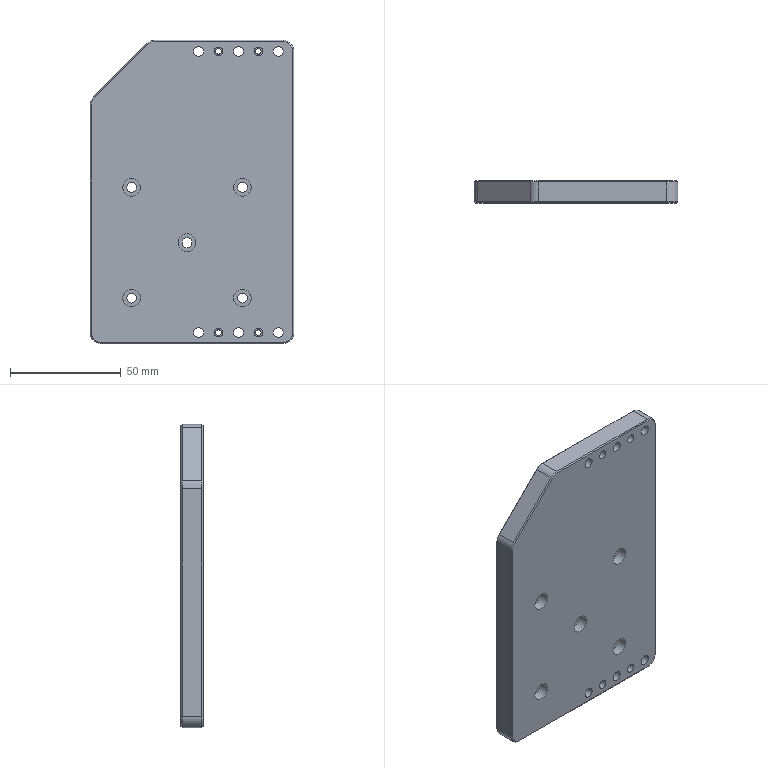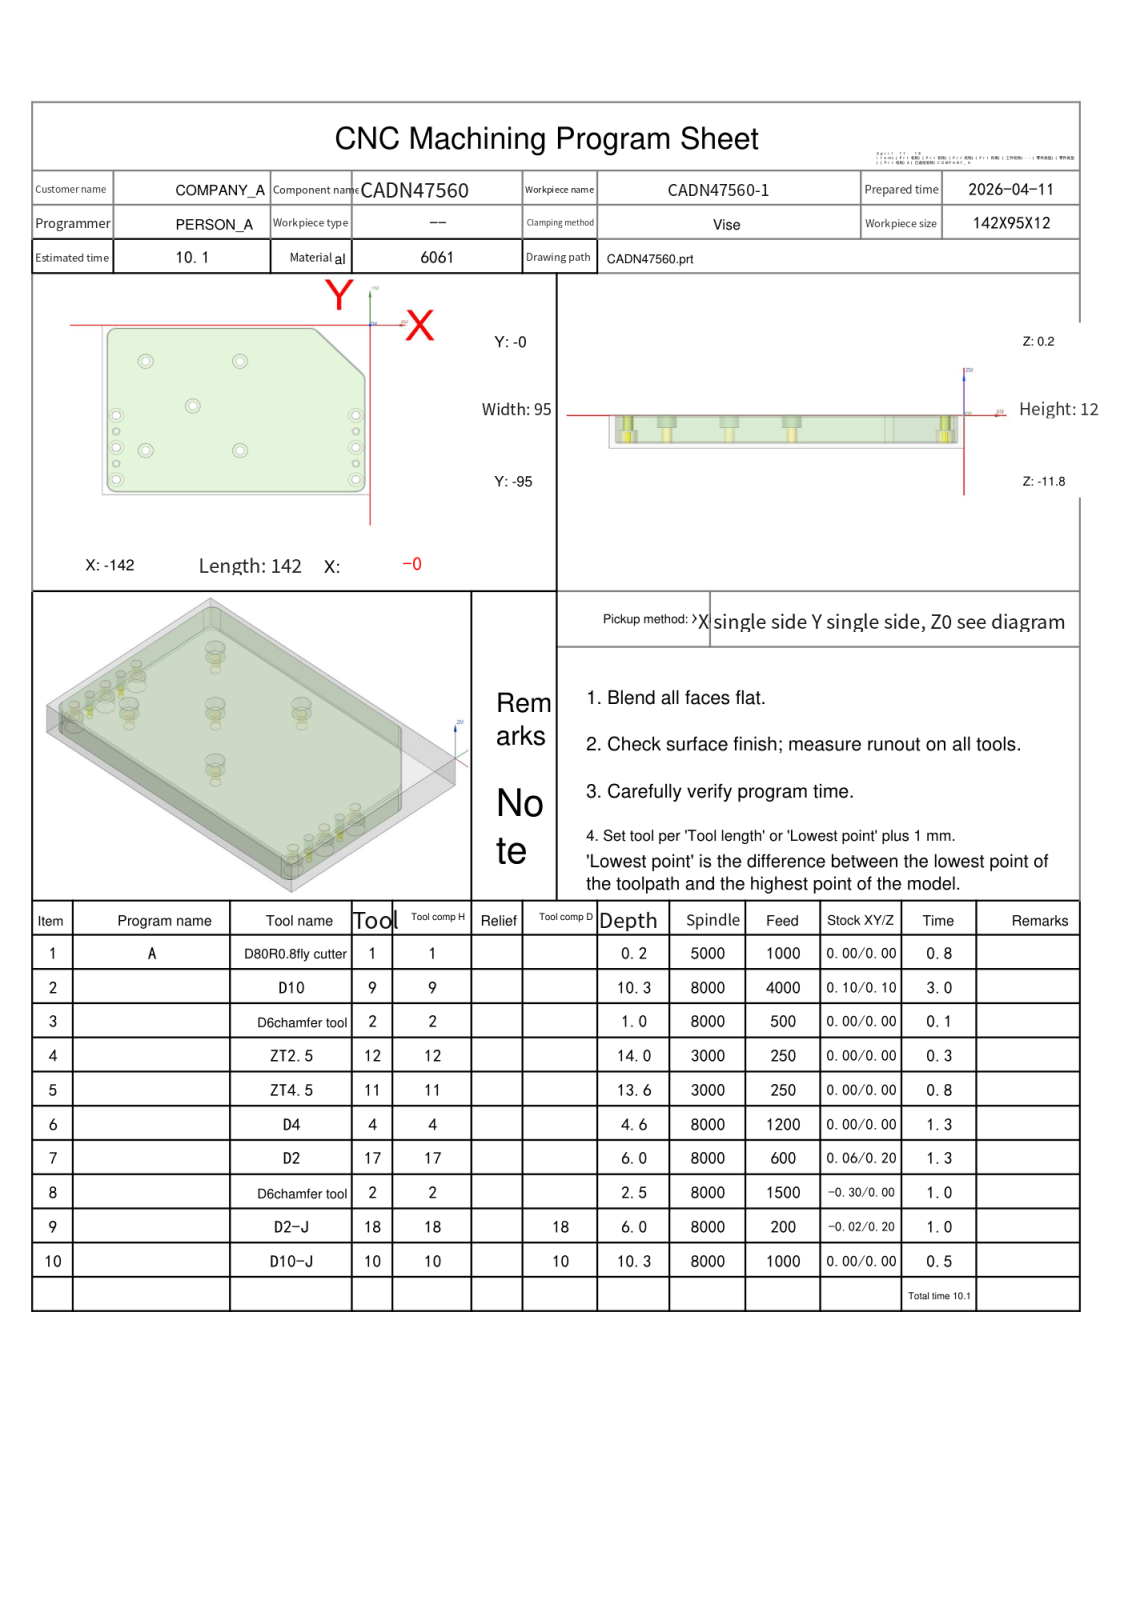NC program | NX | posted by the shop | part box 92 x 10 x 137 mm
Whole program, first 1449 of 1659 lines:
%
O0001
(Machine time: 11.96 MIN)
(===Total Tool:9===)
(T1=D80R0.8 fly cutter D=80.  R=0.8  D-  H01 Z=0.    )
(T9=D10     D=10.  R=0.   D-  H09 Z=-10.1 )
(T2=D6chamfer tool   D=6.   R=0.   D-  H02 Z=-2.3  )
(T12=ZT2.5  D=2.5  DR_a=118 D-  H12 Z=-13.75)
(T11=ZT4.5  D=4.5  DR_a=118 D-  H11 Z=-13.35)
(T4=D4      D=4.   R=0.   D4  H04 Z=-4.4  )
(T17=D2     D=2.   R=0.   D-  H17 Z=-5.8  )
(T18=D2-J   D=2.   R=0.   D18 H18 Z=-5.8  )
(T10=D10-J  D=10.  R=0.   D10 H10 Z=-10.1 )
G80 G90 G17 G49 G40
G91 G28 Z0
M01
N1 T01 M06
(D80R0.8 fly cutter  D=80. R=0.8 H=01 ce=0.00 di=0.00)
G00 G90 G54 X-184.5 Y-4.5 M03 S5000
G43 H01 Z20.
M08
Z2.
G01 Z0.0 F1000.
X-179.5
X37.5
Y-47.5
X-179.5
Y-90.5
X37.5
X42.5
Z2.
G00 Z20.
G91 G28 Z0.0
M05
M09
G91 G28 Z0.0
M01
N2 T09 M06
(D10  D=10. R=0. H=09 ce=0.10 di=0.10)
G00 G90 G54 X-7.906 Y12. M03 S8000
G43 H09 Z10.2
M08
Z.719
G01 Z-.481 F4000.
G03 X-8.213 Y9.95 I6.693 J-2.05
X-6.163 Y5. I7. J0.0
G01 X4.707 Y-5.87
G02 X5. Y-6.576 I-.707 J-.707
G01 Y-16.511
G02 X4.6 Y-16.911 I-.4 J0.0
X4.317 Y-16.794 I0.0 J.4
G01 X-16.864 Y4.388
G03 X-17.571 Y4.681 I-.707 J-.707
X-18.17 Y4.482 I0.0 J-1.
G01 X-23.025 Y.851
G03 X-23.426 Y.05 I.599 J-.801
X-23.133 Y-.657 I1. J0.0
G01 X-.36 Y-23.431
G02 X2.598 Y-30.571 I-7.14 J-7.14
G01 Y-88.5
G02 X-7.5 Y-98.598 I-10.098 J0.0
G01 X-134.5
G02 X-144.598 Y-88.5 I0.0 J10.098
G01 Y-6.5
G02 X-134.5 Y3.598 I10.098 J0.0
G01 X-31.571
G02 X-24.431 Y.64 I0.0 J-10.098
G01 X-19.598 Y-4.192
X-19.244 Y-4.546
G03 X-14.294 Y-6.596 I4.95 J4.95
X-9.345 Y-4.546 I0.0 J7.
G01 Y12.
Z.719
G00 Z3.
G01 X-7.903 F6000.
G00 Z.238
G01 Z-.962 F4000.
G03 X-8.21 Y9.95 I6.693 J-2.05
X-6.16 Y5. I7. J0.0
G01 X4.707 Y-5.867
G02 X5. Y-6.574 I-.707 J-.707
G01 Y-16.508
G02 X4.6 Y-16.908 I-.4 J0.0
X4.317 Y-16.791 I0.0 J.4
G01 X-16.862 Y4.388
G03 X-17.569 Y4.681 I-.707 J-.707
X-18.167 Y4.482 I0.0 J-1.
G01 X-23.022 Y.851
G03 X-23.424 Y.05 I.599 J-.801
X-23.131 Y-.657 I1. J0.0
G01 X-.358 Y-23.429
G02 X2.6 Y-30.571 I-7.142 J-7.142
G01 Y-88.5
G02 X-7.5 Y-98.6 I-10.1 J0.0
G01 X-134.5
G02 X-144.6 Y-88.5 I0.0 J10.1
G01 Y-6.5
G02 X-134.5 Y3.6 I10.1 J0.0
G01 X-31.571
G02 X-24.429 Y.642 I0.0 J-10.1
G01 X-19.595 Y-4.192
X-19.242 Y-4.546
G03 X-14.292 Y-6.596 I4.95 J4.95
X-9.342 Y-4.546 I0.0 J7.
G01 Y12.
Z.238
G00 Z2.519
G01 X-7.903 F6000.
G00 Z-.243
G01 Z-1.443 F4000.
G03 X-8.21 Y9.95 I6.693 J-2.05
X-6.16 Y5. I7. J0.0
G01 X4.707 Y-5.867
G02 X5. Y-6.574 I-.707 J-.707
G01 Y-16.508
G02 X4.6 Y-16.908 I-.4 J0.0
X4.317 Y-16.791 I0.0 J.4
G01 X-16.862 Y4.388
G03 X-17.569 Y4.681 I-.707 J-.707
X-18.167 Y4.482 I0.0 J-1.
G01 X-23.022 Y.851
G03 X-23.424 Y.05 I.599 J-.801
X-23.131 Y-.657 I1. J0.0
G01 X-.358 Y-23.429
G02 X2.6 Y-30.571 I-7.142 J-7.142
G01 Y-88.5
G02 X-7.5 Y-98.6 I-10.1 J0.0
G01 X-134.5
G02 X-144.6 Y-88.5 I0.0 J10.1
G01 Y-6.5
G02 X-134.5 Y3.6 I10.1 J0.0
G01 X-31.571
G02 X-24.429 Y.642 I0.0 J-10.1
G01 X-19.595 Y-4.192
X-19.242 Y-4.546
G03 X-14.292 Y-6.596 I4.95 J4.95
X-9.342 Y-4.546 I0.0 J7.
G01 Y12.
Z-.243
G00 Z2.038
G01 X-7.903 F6000.
G00 Z-.724
G01 Z-1.924 F4000.
G03 X-8.21 Y9.95 I6.693 J-2.05
X-6.16 Y5. I7. J0.0
G01 X4.707 Y-5.867
G02 X5. Y-6.574 I-.707 J-.707
G01 Y-16.508
G02 X4.6 Y-16.908 I-.4 J0.0
X4.317 Y-16.791 I0.0 J.4
G01 X-16.862 Y4.388
G03 X-17.569 Y4.681 I-.707 J-.707
X-18.167 Y4.482 I0.0 J-1.
G01 X-23.022 Y.851
G03 X-23.424 Y.05 I.599 J-.801
X-23.131 Y-.657 I1. J0.0
G01 X-.358 Y-23.429
G02 X2.6 Y-30.571 I-7.142 J-7.142
G01 Y-88.5
G02 X-7.5 Y-98.6 I-10.1 J0.0
G01 X-134.5
G02 X-144.6 Y-88.5 I0.0 J10.1
G01 Y-6.5
G02 X-134.5 Y3.6 I10.1 J0.0
G01 X-31.571
G02 X-24.429 Y.642 I0.0 J-10.1
G01 X-19.595 Y-4.192
X-19.242 Y-4.546
G03 X-14.292 Y-6.596 I4.95 J4.95
X-9.342 Y-4.546 I0.0 J7.
G01 Y12.
Z-.724
G00 Z1.557
G01 X-7.903 F6000.
G00 Z-1.205
G01 Z-2.405 F4000.
G03 X-8.21 Y9.95 I6.693 J-2.05
X-6.16 Y5. I7. J0.0
G01 X4.707 Y-5.867
G02 X5. Y-6.574 I-.707 J-.707
G01 Y-16.508
G02 X4.6 Y-16.908 I-.4 J0.0
X4.317 Y-16.791 I0.0 J.4
G01 X-16.862 Y4.388
G03 X-17.569 Y4.681 I-.707 J-.707
X-18.167 Y4.482 I0.0 J-1.
G01 X-23.022 Y.851
G03 X-23.424 Y.05 I.599 J-.801
X-23.131 Y-.657 I1. J0.0
G01 X-.358 Y-23.429
G02 X2.6 Y-30.571 I-7.142 J-7.142
G01 Y-88.5
G02 X-7.5 Y-98.6 I-10.1 J0.0
G01 X-134.5
G02 X-144.6 Y-88.5 I0.0 J10.1
G01 Y-6.5
G02 X-134.5 Y3.6 I10.1 J0.0
G01 X-31.571
G02 X-24.429 Y.642 I0.0 J-10.1
G01 X-19.595 Y-4.192
X-19.242 Y-4.546
G03 X-14.292 Y-6.596 I4.95 J4.95
X-9.342 Y-4.546 I0.0 J7.
G01 Y12.
Z-1.205
G00 Z1.076
G01 X-7.903 F6000.
G00 Z-1.686
G01 Z-2.886 F4000.
G03 X-8.21 Y9.95 I6.693 J-2.05
X-6.16 Y5. I7. J0.0
G01 X4.707 Y-5.867
G02 X5. Y-6.574 I-.707 J-.707
G01 Y-16.508
G02 X4.6 Y-16.908 I-.4 J0.0
X4.317 Y-16.791 I0.0 J.4
G01 X-16.862 Y4.388
G03 X-17.569 Y4.681 I-.707 J-.707
X-18.167 Y4.482 I0.0 J-1.
G01 X-23.022 Y.851
G03 X-23.424 Y.05 I.599 J-.801
X-23.131 Y-.657 I1. J0.0
G01 X-.358 Y-23.429
G02 X2.6 Y-30.571 I-7.142 J-7.142
G01 Y-88.5
G02 X-7.5 Y-98.6 I-10.1 J0.0
G01 X-134.5
G02 X-144.6 Y-88.5 I0.0 J10.1
G01 Y-6.5
G02 X-134.5 Y3.6 I10.1 J0.0
G01 X-31.571
G02 X-24.429 Y.642 I0.0 J-10.1
G01 X-19.595 Y-4.192
X-19.242 Y-4.546
G03 X-14.292 Y-6.596 I4.95 J4.95
X-9.342 Y-4.546 I0.0 J7.
G01 Y12.
Z-1.686
G00 Z.595
G01 X-7.903 F6000.
G00 Z-2.167
G01 Z-3.367 F4000.
G03 X-8.21 Y9.95 I6.693 J-2.05
X-6.16 Y5. I7. J0.0
G01 X4.707 Y-5.867
G02 X5. Y-6.574 I-.707 J-.707
G01 Y-16.508
G02 X4.6 Y-16.908 I-.4 J0.0
X4.317 Y-16.791 I0.0 J.4
G01 X-16.862 Y4.388
G03 X-17.569 Y4.681 I-.707 J-.707
X-18.167 Y4.482 I0.0 J-1.
G01 X-23.022 Y.851
G03 X-23.424 Y.05 I.599 J-.801
X-23.131 Y-.657 I1. J0.0
G01 X-.358 Y-23.429
G02 X2.6 Y-30.571 I-7.142 J-7.142
G01 Y-88.5
G02 X-7.5 Y-98.6 I-10.1 J0.0
G01 X-134.5
G02 X-144.6 Y-88.5 I0.0 J10.1
G01 Y-6.5
G02 X-134.5 Y3.6 I10.1 J0.0
G01 X-31.571
G02 X-24.429 Y.642 I0.0 J-10.1
G01 X-19.595 Y-4.192
X-19.242 Y-4.546
G03 X-14.292 Y-6.596 I4.95 J4.95
X-9.342 Y-4.546 I0.0 J7.
G01 Y12.
Z-2.167
G00 Z.114
G01 X-7.903 F6000.
G00 Z-2.648
G01 Z-3.848 F4000.
G03 X-8.21 Y9.95 I6.693 J-2.05
X-6.16 Y5. I7. J0.0
G01 X4.707 Y-5.867
G02 X5. Y-6.574 I-.707 J-.707
G01 Y-16.508
G02 X4.6 Y-16.908 I-.4 J0.0
X4.317 Y-16.791 I0.0 J.4
G01 X-16.862 Y4.388
G03 X-17.569 Y4.681 I-.707 J-.707
X-18.167 Y4.482 I0.0 J-1.
G01 X-23.022 Y.851
G03 X-23.424 Y.05 I.599 J-.801
X-23.131 Y-.657 I1. J0.0
G01 X-.358 Y-23.429
G02 X2.6 Y-30.571 I-7.142 J-7.142
G01 Y-88.5
G02 X-7.5 Y-98.6 I-10.1 J0.0
G01 X-134.5
G02 X-144.6 Y-88.5 I0.0 J10.1
G01 Y-6.5
G02 X-134.5 Y3.6 I10.1 J0.0
G01 X-31.571
G02 X-24.429 Y.642 I0.0 J-10.1
G01 X-19.595 Y-4.192
X-19.242 Y-4.546
G03 X-14.292 Y-6.596 I4.95 J4.95
X-9.342 Y-4.546 I0.0 J7.
G01 Y12.
Z-2.648
G00 Z-.367
G01 X-7.903 F6000.
G00 Z-3.129
G01 Z-4.329 F4000.
G03 X-8.21 Y9.95 I6.693 J-2.05
X-6.16 Y5. I7. J0.0
G01 X4.707 Y-5.867
G02 X5. Y-6.574 I-.707 J-.707
G01 Y-16.508
G02 X4.6 Y-16.908 I-.4 J0.0
X4.317 Y-16.791 I0.0 J.4
G01 X-16.862 Y4.388
G03 X-17.569 Y4.681 I-.707 J-.707
X-18.167 Y4.482 I0.0 J-1.
G01 X-23.022 Y.851
G03 X-23.424 Y.05 I.599 J-.801
X-23.131 Y-.657 I1. J0.0
G01 X-.358 Y-23.429
G02 X2.6 Y-30.571 I-7.142 J-7.142
G01 Y-88.5
G02 X-7.5 Y-98.6 I-10.1 J0.0
G01 X-134.5
G02 X-144.6 Y-88.5 I0.0 J10.1
G01 Y-6.5
G02 X-134.5 Y3.6 I10.1 J0.0
G01 X-31.571
G02 X-24.429 Y.642 I0.0 J-10.1
G01 X-19.595 Y-4.192
X-19.242 Y-4.546
G03 X-14.292 Y-6.596 I4.95 J4.95
X-9.342 Y-4.546 I0.0 J7.
G01 Y12.
Z-3.129
G00 Z-.848
G01 X-7.903 F6000.
G00 Z-3.61
G01 Z-4.81 F4000.
G03 X-8.21 Y9.95 I6.693 J-2.05
X-6.16 Y5. I7. J0.0
G01 X4.707 Y-5.867
G02 X5. Y-6.574 I-.707 J-.707
G01 Y-16.508
G02 X4.6 Y-16.908 I-.4 J0.0
X4.317 Y-16.791 I0.0 J.4
G01 X-16.862 Y4.388
G03 X-17.569 Y4.681 I-.707 J-.707
X-18.167 Y4.482 I0.0 J-1.
G01 X-23.022 Y.851
G03 X-23.424 Y.05 I.599 J-.801
X-23.131 Y-.657 I1. J0.0
G01 X-.358 Y-23.429
G02 X2.6 Y-30.571 I-7.142 J-7.142
G01 Y-88.5
G02 X-7.5 Y-98.6 I-10.1 J0.0
G01 X-134.5
G02 X-144.6 Y-88.5 I0.0 J10.1
G01 Y-6.5
G02 X-134.5 Y3.6 I10.1 J0.0
G01 X-31.571
G02 X-24.429 Y.642 I0.0 J-10.1
G01 X-19.595 Y-4.192
X-19.242 Y-4.546
G03 X-14.292 Y-6.596 I4.95 J4.95
X-9.342 Y-4.546 I0.0 J7.
G01 Y12.
Z-3.61
G00 Z-1.329
G01 X-7.903 F6000.
G00 Z-4.09
G01 Z-5.29 F4000.
G03 X-8.21 Y9.95 I6.693 J-2.05
X-6.16 Y5. I7. J0.0
G01 X4.707 Y-5.867
G02 X5. Y-6.574 I-.707 J-.707
G01 Y-16.508
G02 X4.6 Y-16.908 I-.4 J0.0
X4.317 Y-16.791 I0.0 J.4
G01 X-16.862 Y4.388
G03 X-17.569 Y4.681 I-.707 J-.707
X-18.167 Y4.482 I0.0 J-1.
G01 X-23.022 Y.851
G03 X-23.424 Y.05 I.599 J-.801
X-23.131 Y-.657 I1. J0.0
G01 X-.358 Y-23.429
G02 X2.6 Y-30.571 I-7.142 J-7.142
G01 Y-88.5
G02 X-7.5 Y-98.6 I-10.1 J0.0
G01 X-134.5
G02 X-144.6 Y-88.5 I0.0 J10.1
G01 Y-6.5
G02 X-134.5 Y3.6 I10.1 J0.0
G01 X-31.571
G02 X-24.429 Y.642 I0.0 J-10.1
G01 X-19.595 Y-4.192
X-19.242 Y-4.546
G03 X-14.292 Y-6.596 I4.95 J4.95
X-9.342 Y-4.546 I0.0 J7.
G01 Y12.
Z-4.09
G00 Z-1.81
G01 X-7.903 F6000.
G00 Z-4.571
G01 Z-5.771 F4000.
G03 X-8.21 Y9.95 I6.693 J-2.05
X-6.16 Y5. I7. J0.0
G01 X4.707 Y-5.867
G02 X5. Y-6.574 I-.707 J-.707
G01 Y-16.508
G02 X4.6 Y-16.908 I-.4 J0.0
X4.317 Y-16.791 I0.0 J.4
G01 X-16.862 Y4.388
G03 X-17.569 Y4.681 I-.707 J-.707
X-18.167 Y4.482 I0.0 J-1.
G01 X-23.022 Y.851
G03 X-23.424 Y.05 I.599 J-.801
X-23.131 Y-.657 I1. J0.0
G01 X-.358 Y-23.429
G02 X2.6 Y-30.571 I-7.142 J-7.142
G01 Y-88.5
G02 X-7.5 Y-98.6 I-10.1 J0.0
G01 X-134.5
G02 X-144.6 Y-88.5 I0.0 J10.1
G01 Y-6.5
G02 X-134.5 Y3.6 I10.1 J0.0
G01 X-31.571
G02 X-24.429 Y.642 I0.0 J-10.1
G01 X-19.595 Y-4.192
X-19.242 Y-4.546
G03 X-14.292 Y-6.596 I4.95 J4.95
X-9.342 Y-4.546 I0.0 J7.
G01 Y12.
Z-4.571
G00 Z-2.29
G01 X-7.903 F6000.
G00 Z-5.052
G01 Z-6.252 F4000.
G03 X-8.21 Y9.95 I6.693 J-2.05
X-6.16 Y5. I7. J0.0
G01 X4.707 Y-5.867
G02 X5. Y-6.574 I-.707 J-.707
G01 Y-16.508
G02 X4.6 Y-16.908 I-.4 J0.0
X4.317 Y-16.791 I0.0 J.4
G01 X-16.862 Y4.388
G03 X-17.569 Y4.681 I-.707 J-.707
X-18.167 Y4.482 I0.0 J-1.
G01 X-23.022 Y.851
G03 X-23.424 Y.05 I.599 J-.801
X-23.131 Y-.657 I1. J0.0
G01 X-.358 Y-23.429
G02 X2.6 Y-30.571 I-7.142 J-7.142
G01 Y-88.5
G02 X-7.5 Y-98.6 I-10.1 J0.0
G01 X-134.5
G02 X-144.6 Y-88.5 I0.0 J10.1
G01 Y-6.5
G02 X-134.5 Y3.6 I10.1 J0.0
G01 X-31.571
G02 X-24.429 Y.642 I0.0 J-10.1
G01 X-19.595 Y-4.192
X-19.242 Y-4.546
G03 X-14.292 Y-6.596 I4.95 J4.95
X-9.342 Y-4.546 I0.0 J7.
G01 Y12.
Z-5.052
G00 Z-2.771
G01 X-7.903 F6000.
G00 Z-5.533
G01 Z-6.733 F4000.
G03 X-8.21 Y9.95 I6.693 J-2.05
X-6.16 Y5. I7. J0.0
G01 X4.707 Y-5.867
G02 X5. Y-6.574 I-.707 J-.707
G01 Y-16.508
G02 X4.6 Y-16.908 I-.4 J0.0
X4.317 Y-16.791 I0.0 J.4
G01 X-16.862 Y4.388
G03 X-17.569 Y4.681 I-.707 J-.707
X-18.167 Y4.482 I0.0 J-1.
G01 X-23.022 Y.851
G03 X-23.424 Y.05 I.599 J-.801
X-23.131 Y-.657 I1. J0.0
G01 X-.358 Y-23.429
G02 X2.6 Y-30.571 I-7.142 J-7.142
G01 Y-88.5
G02 X-7.5 Y-98.6 I-10.1 J0.0
G01 X-134.5
G02 X-144.6 Y-88.5 I0.0 J10.1
G01 Y-6.5
G02 X-134.5 Y3.6 I10.1 J0.0
G01 X-31.571
G02 X-24.429 Y.642 I0.0 J-10.1
G01 X-19.595 Y-4.192
X-19.242 Y-4.546
G03 X-14.292 Y-6.596 I4.95 J4.95
X-9.342 Y-4.546 I0.0 J7.
G01 Y12.
Z-5.533
G00 Z-3.252
G01 X-7.903 F6000.
G00 Z-6.014
G01 Z-7.214 F4000.
G03 X-8.21 Y9.95 I6.693 J-2.05
X-6.16 Y5. I7. J0.0
G01 X4.707 Y-5.867
G02 X5. Y-6.574 I-.707 J-.707
G01 Y-16.508
G02 X4.6 Y-16.908 I-.4 J0.0
X4.317 Y-16.791 I0.0 J.4
G01 X-16.862 Y4.388
G03 X-17.569 Y4.681 I-.707 J-.707
X-18.167 Y4.482 I0.0 J-1.
G01 X-23.022 Y.851
G03 X-23.424 Y.05 I.599 J-.801
X-23.131 Y-.657 I1. J0.0
G01 X-.358 Y-23.429
G02 X2.6 Y-30.571 I-7.142 J-7.142
G01 Y-88.5
G02 X-7.5 Y-98.6 I-10.1 J0.0
G01 X-134.5
G02 X-144.6 Y-88.5 I0.0 J10.1
G01 Y-6.5
G02 X-134.5 Y3.6 I10.1 J0.0
G01 X-31.571
G02 X-24.429 Y.642 I0.0 J-10.1
G01 X-19.595 Y-4.192
X-19.242 Y-4.546
G03 X-14.292 Y-6.596 I4.95 J4.95
X-9.342 Y-4.546 I0.0 J7.
G01 Y12.
Z-6.014
G00 Z-3.733
G01 X-7.903 F6000.
G00 Z-6.495
G01 Z-7.695 F4000.
G03 X-8.21 Y9.95 I6.693 J-2.05
X-6.16 Y5. I7. J0.0
G01 X4.707 Y-5.867
G02 X5. Y-6.574 I-.707 J-.707
G01 Y-16.508
G02 X4.6 Y-16.908 I-.4 J0.0
X4.317 Y-16.791 I0.0 J.4
G01 X-16.862 Y4.388
G03 X-17.569 Y4.681 I-.707 J-.707
X-18.167 Y4.482 I0.0 J-1.
G01 X-23.022 Y.851
G03 X-23.424 Y.05 I.599 J-.801
X-23.131 Y-.657 I1. J0.0
G01 X-.358 Y-23.429
G02 X2.6 Y-30.571 I-7.142 J-7.142
G01 Y-88.5
G02 X-7.5 Y-98.6 I-10.1 J0.0
G01 X-134.5
G02 X-144.6 Y-88.5 I0.0 J10.1
G01 Y-6.5
G02 X-134.5 Y3.6 I10.1 J0.0
G01 X-31.571
G02 X-24.429 Y.642 I0.0 J-10.1
G01 X-19.595 Y-4.192
X-19.242 Y-4.546
G03 X-14.292 Y-6.596 I4.95 J4.95
X-9.342 Y-4.546 I0.0 J7.
G01 Y12.
Z-6.495
G00 Z-4.214
G01 X-7.903 F6000.
G00 Z-6.976
G01 Z-8.176 F4000.
G03 X-8.21 Y9.95 I6.693 J-2.05
X-6.16 Y5. I7. J0.0
G01 X4.707 Y-5.867
G02 X5. Y-6.574 I-.707 J-.707
G01 Y-16.508
G02 X4.6 Y-16.908 I-.4 J0.0
X4.317 Y-16.791 I0.0 J.4
G01 X-16.862 Y4.388
G03 X-17.569 Y4.681 I-.707 J-.707
X-18.167 Y4.482 I0.0 J-1.
G01 X-23.022 Y.851
G03 X-23.424 Y.05 I.599 J-.801
X-23.131 Y-.657 I1. J0.0
G01 X-.358 Y-23.429
G02 X2.6 Y-30.571 I-7.142 J-7.142
G01 Y-88.5
G02 X-7.5 Y-98.6 I-10.1 J0.0
G01 X-134.5
G02 X-144.6 Y-88.5 I0.0 J10.1
G01 Y-6.5
G02 X-134.5 Y3.6 I10.1 J0.0
G01 X-31.571
G02 X-24.429 Y.642 I0.0 J-10.1
G01 X-19.595 Y-4.192
X-19.242 Y-4.546
G03 X-14.292 Y-6.596 I4.95 J4.95
X-9.342 Y-4.546 I0.0 J7.
G01 Y12.
Z-6.976
G00 Z-4.695
G01 X-7.903 F6000.
G00 Z-7.457
G01 Z-8.657 F4000.
G03 X-8.21 Y9.95 I6.693 J-2.05
X-6.16 Y5. I7. J0.0
G01 X4.707 Y-5.867
G02 X5. Y-6.574 I-.707 J-.707
G01 Y-16.508
G02 X4.6 Y-16.908 I-.4 J0.0
X4.317 Y-16.791 I0.0 J.4
G01 X-16.862 Y4.388
G03 X-17.569 Y4.681 I-.707 J-.707
X-18.167 Y4.482 I0.0 J-1.
G01 X-23.022 Y.851
G03 X-23.424 Y.05 I.599 J-.801
X-23.131 Y-.657 I1. J0.0
G01 X-.358 Y-23.429
G02 X2.6 Y-30.571 I-7.142 J-7.142
G01 Y-88.5
G02 X-7.5 Y-98.6 I-10.1 J0.0
G01 X-134.5
G02 X-144.6 Y-88.5 I0.0 J10.1
G01 Y-6.5
G02 X-134.5 Y3.6 I10.1 J0.0
G01 X-31.571
G02 X-24.429 Y.642 I0.0 J-10.1
G01 X-19.595 Y-4.192
X-19.242 Y-4.546
G03 X-14.292 Y-6.596 I4.95 J4.95
X-9.342 Y-4.546 I0.0 J7.
G01 Y12.
Z-7.457
G00 Z-5.176
G01 X-7.903 F6000.
G00 Z-7.938
G01 Z-9.138 F4000.
G03 X-8.21 Y9.95 I6.693 J-2.05
X-6.16 Y5. I7. J0.0
G01 X4.707 Y-5.867
G02 X5. Y-6.574 I-.707 J-.707
G01 Y-16.508
G02 X4.6 Y-16.908 I-.4 J0.0
X4.317 Y-16.791 I0.0 J.4
G01 X-16.862 Y4.388
G03 X-17.569 Y4.681 I-.707 J-.707
X-18.167 Y4.482 I0.0 J-1.
G01 X-23.022 Y.851
G03 X-23.424 Y.05 I.599 J-.801
X-23.131 Y-.657 I1. J0.0
G01 X-.358 Y-23.429
G02 X2.6 Y-30.571 I-7.142 J-7.142
G01 Y-88.5
G02 X-7.5 Y-98.6 I-10.1 J0.0
G01 X-134.5
G02 X-144.6 Y-88.5 I0.0 J10.1
G01 Y-6.5
G02 X-134.5 Y3.6 I10.1 J0.0
G01 X-31.571
G02 X-24.429 Y.642 I0.0 J-10.1
G01 X-19.595 Y-4.192
X-19.242 Y-4.546
G03 X-14.292 Y-6.596 I4.95 J4.95
X-9.342 Y-4.546 I0.0 J7.
G01 Y12.
Z-7.938
G00 Z-5.657
G01 X-7.903 F6000.
G00 Z-8.419
G01 Z-9.619 F4000.
G03 X-8.21 Y9.95 I6.693 J-2.05
X-6.16 Y5. I7. J0.0
G01 X4.707 Y-5.867
G02 X5. Y-6.574 I-.707 J-.707
G01 Y-16.508
G02 X4.6 Y-16.908 I-.4 J0.0
X4.317 Y-16.791 I0.0 J.4
G01 X-16.862 Y4.388
G03 X-17.569 Y4.681 I-.707 J-.707
X-18.167 Y4.482 I0.0 J-1.
G01 X-23.022 Y.851
G03 X-23.424 Y.05 I.599 J-.801
X-23.131 Y-.657 I1. J0.0
G01 X-.358 Y-23.429
G02 X2.6 Y-30.571 I-7.142 J-7.142
G01 Y-88.5
G02 X-7.5 Y-98.6 I-10.1 J0.0
G01 X-134.5
G02 X-144.6 Y-88.5 I0.0 J10.1
G01 Y-6.5
G02 X-134.5 Y3.6 I10.1 J0.0
G01 X-31.571
G02 X-24.429 Y.642 I0.0 J-10.1
G01 X-19.595 Y-4.192
X-19.242 Y-4.546
G03 X-14.292 Y-6.596 I4.95 J4.95
X-9.342 Y-4.546 I0.0 J7.
G01 Y12.
Z-8.419
G00 Z-6.138
G01 X-7.903 F6000.
G00 Z-8.9
G01 Z-10.1 F4000.
G03 X-8.21 Y9.95 I6.693 J-2.05
X-6.16 Y5. I7. J0.0
G01 X4.707 Y-5.867
G02 X5. Y-6.574 I-.707 J-.707
G01 Y-16.508
G02 X4.6 Y-16.908 I-.4 J0.0
X4.317 Y-16.791 I0.0 J.4
G01 X-16.862 Y4.388
G03 X-17.569 Y4.681 I-.707 J-.707
X-18.167 Y4.482 I0.0 J-1.
G01 X-23.022 Y.851
G03 X-23.424 Y.05 I.599 J-.801
X-23.131 Y-.657 I1. J0.0
G01 X-.358 Y-23.429
G02 X2.6 Y-30.571 I-7.142 J-7.142
G01 Y-88.5
G02 X-7.5 Y-98.6 I-10.1 J0.0
G01 X-134.5
G02 X-144.6 Y-88.5 I0.0 J10.1
G01 Y-6.5
G02 X-134.5 Y3.6 I10.1 J0.0
G01 X-31.571
G02 X-24.429 Y.642 I0.0 J-10.1
G01 X-19.595 Y-4.192
X-19.242 Y-4.546
G03 X-14.292 Y-6.596 I4.95 J4.95
X-9.342 Y-4.546 I0.0 J7.
G01 Y12.
Z-8.9
G00 Z10.2
G91 G28 Z0.0
M05
M09
G91 G28 Z0.0
M01
N3 T02 M06
(D6chamfer tool  D=6. R=0. H=02 ce=0.00 di=0.10)
G00 G90 G54 X-7.5 Y-50.5 M03 S8000
G43 H02 Z20.
M08
G98 G81 X-7.5 Y-50.5 Z-.8 R1. F500.
Y-59.5
Y-68.5
Y-77.5
Y-86.5
X-68.901 Y-70.25
Y-20.25
X-93.901 Y-45.25
X-118.901 Y-20.25
X-134.5 Y-50.5
Y-59.5
Y-68.5
Y-77.5
Y-86.5
X-118.901 Y-70.25
G80
G00 Z20.
G91 G28 Z0.0
M05
M09
G91 G28 Z0.0
M01
N4 T12 M06
(ZT2.5 D=2.5 DR_a=118 H=12)
G00 G90 G54 X-134.5 Y-59.5 M03 S3000
G43 H12 Z20.
M08
G98 G83 X-134.5 Y-59.5 Z-13.751 R1. F250. Q2.
Y-77.5
X-7.5
Y-59.5
G80
G00 Z20.
G91 G28 Z0.0
M05
M09
G91 G28 Z0.0
M01
N5 T11 M06
(ZT4.5 D=4.5 DR_a=118 H=11)
G00 G90 G54 X-7.5 Y-86.5 M03 S3000
G43 H11 Z20.
M08
G98 G83 X-7.5 Y-86.5 Z-13. R1. F250. Q3.
Y-68.5
Y-50.5
X-134.5
Y-68.5
Y-86.5
G80
G00 Z20.
G00 G90 X-118.901 Y-20.25 M03 S2800
Z20.
G98 G83 X-118.901 Y-20.25 Z-13.352 R1. F200. Q2.
X-68.901
Y-70.25
X-93.901 Y-45.25
X-118.901 Y-70.25
G80
G00 Z20.
G91 G28 Z0.0
M05
M09
G91 G28 Z0.0
M01
N6 T04 M06
(D4  D=4. R=0. H=04 ce=0.10 di=0.00)
G00 G90 G54 X-93.901 Y-45.25 M03 S8000
G43 H04 Z20.
M08
Z.5
G03 X-94.851 Y-46.2 I0.0 J-.95 F1200.
X-93.901 Y-47.15 I.95 J0.0
X-93.901 Y-47.15 Z.2 I0.0 J1.9
X-93.901 Y-47.15 Z-.1 I0.0 J1.9
X-93.901 Y-47.15 Z-.4 I0.0 J1.9
X-93.901 Y-47.15 Z-.7 I0.0 J1.9
X-93.901 Y-47.15 Z-1. I0.0 J1.9
X-93.901 Y-47.15 Z-1.3 I0.0 J1.9
X-93.901 Y-47.15 Z-1.6 I0.0 J1.9
X-93.901 Y-47.15 Z-1.9 I0.0 J1.9
X-93.901 Y-47.15 Z-2.2 I0.0 J1.9
X-93.901 Y-47.15 Z-2.5 I0.0 J1.9
X-93.901 Y-47.15 Z-2.8 I0.0 J1.9
X-93.901 Y-47.15 Z-3.1 I0.0 J1.9
X-93.901 Y-47.15 Z-3.4 I0.0 J1.9
X-93.901 Y-47.15 Z-3.7 I0.0 J1.9
X-93.901 Y-47.15 Z-4. I0.0 J1.9
X-93.901 Y-47.15 Z-4.3 I0.0 J1.9
X-92.256 Y-44.3 Z-4.4 I0.0 J1.9
X-93.901 Y-43.35 I-1.645 J-.95
X-95.801 Y-45.25 I0.0 J-1.9
X-93.901 Y-47.15 I1.9 J0.0
X-92.001 Y-45.25 I0.0 J1.9
X-92.256 Y-44.3 I-1.9 J0.0
X-93.078 Y-43.825 I-.823 J-.475
X-94.028 Y-44.775 I0.0 J-.95
X-93.901 Y-45.25 I.95 J0.0
G00 Z20.
X-118.901 Y-70.25
Z.5
G03 X-119.851 Y-71.2 I0.0 J-.95
X-118.901 Y-72.15 I.95 J0.0
X-118.901 Y-72.15 Z.2 I0.0 J1.9
X-118.901 Y-72.15 Z-.1 I0.0 J1.9
X-118.901 Y-72.15 Z-.4 I0.0 J1.9
X-118.901 Y-72.15 Z-.7 I0.0 J1.9
X-118.901 Y-72.15 Z-1. I0.0 J1.9
X-118.901 Y-72.15 Z-1.3 I0.0 J1.9
X-118.901 Y-72.15 Z-1.6 I0.0 J1.9
X-118.901 Y-72.15 Z-1.9 I0.0 J1.9
X-118.901 Y-72.15 Z-2.2 I0.0 J1.9
X-118.901 Y-72.15 Z-2.5 I0.0 J1.9
X-118.901 Y-72.15 Z-2.8 I0.0 J1.9
X-118.901 Y-72.15 Z-3.1 I0.0 J1.9
X-118.901 Y-72.15 Z-3.4 I0.0 J1.9
X-118.901 Y-72.15 Z-3.7 I0.0 J1.9
X-118.901 Y-72.15 Z-4. I0.0 J1.9
X-118.901 Y-72.15 Z-4.3 I0.0 J1.9
X-117.256 Y-69.3 Z-4.4 I0.0 J1.9
X-118.901 Y-68.35 I-1.645 J-.95
X-120.801 Y-70.25 I0.0 J-1.9
X-118.901 Y-72.15 I1.9 J0.0
X-117.001 Y-70.25 I0.0 J1.9
X-117.256 Y-69.3 I-1.9 J0.0
X-118.078 Y-68.825 I-.823 J-.475
X-119.028 Y-69.775 I0.0 J-.95
X-118.901 Y-70.25 I.95 J0.0
G00 Z20.
X-68.901
Z.5
G03 X-69.851 Y-71.2 I0.0 J-.95
X-68.901 Y-72.15 I.95 J0.0
X-68.901 Y-72.15 Z.2 I0.0 J1.9
X-68.901 Y-72.15 Z-.1 I0.0 J1.9
X-68.901 Y-72.15 Z-.4 I0.0 J1.9
X-68.901 Y-72.15 Z-.7 I0.0 J1.9
X-68.901 Y-72.15 Z-1. I0.0 J1.9
X-68.901 Y-72.15 Z-1.3 I0.0 J1.9
X-68.901 Y-72.15 Z-1.6 I0.0 J1.9
X-68.901 Y-72.15 Z-1.9 I0.0 J1.9
X-68.901 Y-72.15 Z-2.2 I0.0 J1.9
X-68.901 Y-72.15 Z-2.5 I0.0 J1.9
X-68.901 Y-72.15 Z-2.8 I0.0 J1.9
X-68.901 Y-72.15 Z-3.1 I0.0 J1.9
X-68.901 Y-72.15 Z-3.4 I0.0 J1.9
X-68.901 Y-72.15 Z-3.7 I0.0 J1.9
X-68.901 Y-72.15 Z-4. I0.0 J1.9
X-68.901 Y-72.15 Z-4.3 I0.0 J1.9
X-67.256 Y-69.3 Z-4.4 I0.0 J1.9
X-68.901 Y-68.35 I-1.645 J-.95
X-70.801 Y-70.25 I0.0 J-1.9
X-68.901 Y-72.15 I1.9 J0.0
X-67.001 Y-70.25 I0.0 J1.9
X-67.256 Y-69.3 I-1.9 J0.0
X-68.078 Y-68.825 I-.823 J-.475
X-69.028 Y-69.775 I0.0 J-.95
X-68.901 Y-70.25 I.95 J0.0
G00 Z20.
Y-20.25
Z.5
G03 X-69.851 Y-21.2 I0.0 J-.95
X-68.901 Y-22.15 I.95 J0.0
X-68.901 Y-22.15 Z.2 I0.0 J1.9
X-68.901 Y-22.15 Z-.1 I0.0 J1.9
X-68.901 Y-22.15 Z-.4 I0.0 J1.9
X-68.901 Y-22.15 Z-.7 I0.0 J1.9
X-68.901 Y-22.15 Z-1. I0.0 J1.9
X-68.901 Y-22.15 Z-1.3 I0.0 J1.9
X-68.901 Y-22.15 Z-1.6 I0.0 J1.9
X-68.901 Y-22.15 Z-1.9 I0.0 J1.9
X-68.901 Y-22.15 Z-2.2 I0.0 J1.9
X-68.901 Y-22.15 Z-2.5 I0.0 J1.9
X-68.901 Y-22.15 Z-2.8 I0.0 J1.9
X-68.901 Y-22.15 Z-3.1 I0.0 J1.9
X-68.901 Y-22.15 Z-3.4 I0.0 J1.9
X-68.901 Y-22.15 Z-3.7 I0.0 J1.9
X-68.901 Y-22.15 Z-4. I0.0 J1.9
X-68.901 Y-22.15 Z-4.3 I0.0 J1.9
X-67.256 Y-19.3 Z-4.4 I0.0 J1.9
X-68.901 Y-18.35 I-1.645 J-.95
X-70.801 Y-20.25 I0.0 J-1.9
X-68.901 Y-22.15 I1.9 J0.0
X-67.001 Y-20.25 I0.0 J1.9
X-67.256 Y-19.3 I-1.9 J0.0
X-68.078 Y-18.825 I-.823 J-.475
X-69.028 Y-19.775 I0.0 J-.95
X-68.901 Y-20.25 I.95 J0.0
G00 Z20.
X-118.901
Z.5
G03 X-119.851 Y-21.2 I0.0 J-.95
X-118.901 Y-22.15 I.95 J0.0
X-118.901 Y-22.15 Z.2 I0.0 J1.9
X-118.901 Y-22.15 Z-.1 I0.0 J1.9
X-118.901 Y-22.15 Z-.4 I0.0 J1.9
X-118.901 Y-22.15 Z-.7 I0.0 J1.9
X-118.901 Y-22.15 Z-1. I0.0 J1.9
X-118.901 Y-22.15 Z-1.3 I0.0 J1.9
X-118.901 Y-22.15 Z-1.6 I0.0 J1.9
X-118.901 Y-22.15 Z-1.9 I0.0 J1.9
X-118.901 Y-22.15 Z-2.2 I0.0 J1.9
X-118.901 Y-22.15 Z-2.5 I0.0 J1.9
X-118.901 Y-22.15 Z-2.8 I0.0 J1.9
X-118.901 Y-22.15 Z-3.1 I0.0 J1.9
X-118.901 Y-22.15 Z-3.4 I0.0 J1.9
X-118.901 Y-22.15 Z-3.7 I0.0 J1.9
X-118.901 Y-22.15 Z-4. I0.0 J1.9
X-118.901 Y-22.15 Z-4.3 I0.0 J1.9
X-117.256 Y-19.3 Z-4.4 I0.0 J1.9
X-118.901 Y-18.35 I-1.645 J-.95
X-120.801 Y-20.25 I0.0 J-1.9
X-118.901 Y-22.15 I1.9 J0.0
X-117.001 Y-20.25 I0.0 J1.9
X-117.256 Y-19.3 I-1.9 J0.0
X-118.078 Y-18.825 I-.823 J-.475
X-119.028 Y-19.775 I0.0 J-.95
X-118.901 Y-20.25 I.95 J0.0
G00 Z20.
G00 G90 X-93.901 Y-45.25 M03 S8000
Z20.
Z.5
G41 D04
G01 X-94.097 Y-45.29 F500.
G03 X-94.891 Y-46.26 I.196 J-.97
X-93.901 Y-47.25 I.99 J0.0
X-94.152 Y-47.234 Z-4.4 I0.0 J2.
X-93.901 Y-47.25 I.251 J1.984
X-91.901 Y-45.25 I0.0 J2.
X-93.901 Y-43.25 I-2. J0.0
X-95.901 Y-45.25 I0.0 J-2.
X-94.152 Y-47.234 I2. J0.0
G01 X-94.028 Y-47.242
G03 X-93.038 Y-46.252 I0.0 J.99
X-93.711 Y-45.314 I-.99 J0.0
G01 G40 X-93.901 Y-45.25
G00 Z20.
X-118.901 Y-70.25
Z.5
G41 D04
G01 X-119.097 Y-70.29
G03 X-119.891 Y-71.26 I.196 J-.97
X-118.901 Y-72.25 I.99 J0.0
X-119.152 Y-72.234 Z-4.4 I0.0 J2.
X-118.901 Y-72.25 I.251 J1.984
X-116.901 Y-70.25 I0.0 J2.
X-118.901 Y-68.25 I-2. J0.0
X-120.901 Y-70.25 I0.0 J-2.
X-119.152 Y-72.234 I2. J0.0
G01 X-119.028 Y-72.242
G03 X-118.038 Y-71.252 I0.0 J.99
X-118.711 Y-70.314 I-.99 J0.0
G01 G40 X-118.901 Y-70.25
G00 Z20.
X-68.901
Z.5
G41 D04
G01 X-69.097 Y-70.29
G03 X-69.891 Y-71.26 I.196 J-.97
X-68.901 Y-72.25 I.99 J0.0
X-69.152 Y-72.234 Z-4.4 I0.0 J2.
X-68.901 Y-72.25 I.251 J1.984
X-66.901 Y-70.25 I0.0 J2.
X-68.901 Y-68.25 I-2. J0.0
X-70.901 Y-70.25 I0.0 J-2.
X-69.152 Y-72.234 I2. J0.0
G01 X-69.028 Y-72.242
G03 X-68.038 Y-71.252 I0.0 J.99
X-68.711 Y-70.314 I-.99 J0.0
G01 G40 X-68.901 Y-70.25
G00 Z20.
Y-20.25
Z.5
G41 D04
G01 X-69.097 Y-20.29
G03 X-69.891 Y-21.26 I.196 J-.97
X-68.901 Y-22.25 I.99 J0.0
X-69.152 Y-22.234 Z-4.4 I0.0 J2.
X-68.901 Y-22.25 I.251 J1.984
X-66.901 Y-20.25 I0.0 J2.
X-68.901 Y-18.25 I-2. J0.0
X-70.901 Y-20.25 I0.0 J-2.
X-69.152 Y-22.234 I2. J0.0
G01 X-69.028 Y-22.242
G03 X-68.038 Y-21.252 I0.0 J.99
X-68.711 Y-20.314 I-.99 J0.0
G01 G40 X-68.901 Y-20.25
G00 Z20.
X-118.901
Z.5
G41 D04
G01 X-119.097 Y-20.29
G03 X-119.891 Y-21.26 I.196 J-.97
X-118.901 Y-22.25 I.99 J0.0
X-119.152 Y-22.234 Z-4.4 I0.0 J2.
X-118.901 Y-22.25 I.251 J1.984
X-116.901 Y-20.25 I0.0 J2.
X-118.901 Y-18.25 I-2. J0.0
X-120.901 Y-20.25 I0.0 J-2.
X-119.152 Y-22.234 I2. J0.0
G01 X-119.028 Y-22.242
G03 X-118.038 Y-21.252 I0.0 J.99
X-118.711 Y-20.314 I-.99 J0.0
G01 G40 X-118.901 Y-20.25
G00 Z20.
G91 G28 Z0.0
M05
M09
G91 G28 Z0.0
M01
N7 T17 M06
(D2  D=2. R=0. H=17 ce=0.06 di=0.20)
G00 G90 G54 X-134.5 Y-59.5 M03 S8000
G43 H17 Z20.
M08
Z.5
G03 X-134.97 Y-59.97 I0.0 J-.47 F600.
X-134.5 Y-60.44 I.47 J0.0
X-134.5 Y-60.44 Z.3 I0.0 J.94
X-134.5 Y-60.44 Z.1 I0.0 J.94
X-134.5 Y-60.44 Z-.1 I0.0 J.94
X-134.5 Y-60.44 Z-.3 I0.0 J.94
X-134.5 Y-60.44 Z-.5 I0.0 J.94
X-134.5 Y-60.44 Z-.7 I0.0 J.94
X-134.5 Y-60.44 Z-.9 I0.0 J.94
X-134.5 Y-60.44 Z-1.1 I0.0 J.94
X-134.5 Y-60.44 Z-1.3 I0.0 J.94
X-134.5 Y-60.44 Z-1.5 I0.0 J.94
X-134.5 Y-60.44 Z-1.7 I0.0 J.94
X-134.5 Y-60.44 Z-1.9 I0.0 J.94
X-134.5 Y-60.44 Z-2.1 I0.0 J.94
X-134.5 Y-60.44 Z-2.3 I0.0 J.94
X-134.5 Y-60.44 Z-2.5 I0.0 J.94
X-134.5 Y-60.44 Z-2.7 I0.0 J.94
X-134.5 Y-60.44 Z-2.9 I0.0 J.94
X-134.5 Y-60.44 Z-3.1 I0.0 J.94
X-134.5 Y-60.44 Z-3.3 I0.0 J.94
X-134.5 Y-60.44 Z-3.5 I0.0 J.94
X-134.5 Y-60.44 Z-3.7 I0.0 J.94
X-134.5 Y-60.44 Z-3.9 I0.0 J.94
X-134.5 Y-60.44 Z-4.1 I0.0 J.94
X-134.5 Y-60.44 Z-4.3 I0.0 J.94
X-134.5 Y-60.44 Z-4.5 I0.0 J.94
X-134.5 Y-60.44 Z-4.7 I0.0 J.94
X-134.5 Y-60.44 Z-4.9 I0.0 J.94
X-134.5 Y-60.44 Z-5.1 I0.0 J.94
X-134.5 Y-60.44 Z-5.3 I0.0 J.94
X-134.5 Y-60.44 Z-5.5 I0.0 J.94
X-134.5 Y-60.44 Z-5.7 I0.0 J.94
X-134.5 Y-58.56 Z-5.8 I0.0 J.94
X-135.44 Y-59.5 I0.0 J-.94
X-134.5 Y-60.44 I.94 J0.0
X-133.56 Y-59.5 I0.0 J.94
X-134.5 Y-58.56 I-.94 J0.0
X-134.97 Y-59.03 I0.0 J-.47
X-134.5 Y-59.5 I.47 J0.0
G00 Z20.
Y-77.5
Z.5
G03 X-134.97 Y-77.97 I0.0 J-.47
X-134.5 Y-78.44 I.47 J0.0
X-134.5 Y-78.44 Z.3 I0.0 J.94
X-134.5 Y-78.44 Z.1 I0.0 J.94
X-134.5 Y-78.44 Z-.1 I0.0 J.94
X-134.5 Y-78.44 Z-.3 I0.0 J.94
X-134.5 Y-78.44 Z-.5 I0.0 J.94
X-134.5 Y-78.44 Z-.7 I0.0 J.94
X-134.5 Y-78.44 Z-.9 I0.0 J.94
X-134.5 Y-78.44 Z-1.1 I0.0 J.94
X-134.5 Y-78.44 Z-1.3 I0.0 J.94
X-134.5 Y-78.44 Z-1.5 I0.0 J.94
X-134.5 Y-78.44 Z-1.7 I0.0 J.94
X-134.5 Y-78.44 Z-1.9 I0.0 J.94
X-134.5 Y-78.44 Z-2.1 I0.0 J.94
X-134.5 Y-78.44 Z-2.3 I0.0 J.94
X-134.5 Y-78.44 Z-2.5 I0.0 J.94
X-134.5 Y-78.44 Z-2.7 I0.0 J.94
X-134.5 Y-78.44 Z-2.9 I0.0 J.94
X-134.5 Y-78.44 Z-3.1 I0.0 J.94
X-134.5 Y-78.44 Z-3.3 I0.0 J.94
X-134.5 Y-78.44 Z-3.5 I0.0 J.94
X-134.5 Y-78.44 Z-3.7 I0.0 J.94
X-134.5 Y-78.44 Z-3.9 I0.0 J.94
X-134.5 Y-78.44 Z-4.1 I0.0 J.94
X-134.5 Y-78.44 Z-4.3 I0.0 J.94
X-134.5 Y-78.44 Z-4.5 I0.0 J.94
X-134.5 Y-78.44 Z-4.7 I0.0 J.94
X-134.5 Y-78.44 Z-4.9 I0.0 J.94
X-134.5 Y-78.44 Z-5.1 I0.0 J.94
X-134.5 Y-78.44 Z-5.3 I0.0 J.94
X-134.5 Y-78.44 Z-5.5 I0.0 J.94
X-134.5 Y-78.44 Z-5.7 I0.0 J.94
X-134.5 Y-76.56 Z-5.8 I0.0 J.94
X-135.44 Y-77.5 I0.0 J-.94
X-134.5 Y-78.44 I.94 J0.0
X-133.56 Y-77.5 I0.0 J.94
X-134.5 Y-76.56 I-.94 J0.0
X-134.97 Y-77.03 I0.0 J-.47
X-134.5 Y-77.5 I.47 J0.0
G00 Z20.
X-7.5
Z.5
G03 X-7.97 Y-77.97 I0.0 J-.47
X-7.5 Y-78.44 I.47 J0.0
X-7.5 Y-78.44 Z.3 I0.0 J.94
X-7.5 Y-78.44 Z.1 I0.0 J.94
X-7.5 Y-78.44 Z-.1 I0.0 J.94
X-7.5 Y-78.44 Z-.3 I0.0 J.94
X-7.5 Y-78.44 Z-.5 I0.0 J.94
X-7.5 Y-78.44 Z-.7 I0.0 J.94
X-7.5 Y-78.44 Z-.9 I0.0 J.94
X-7.5 Y-78.44 Z-1.1 I0.0 J.94
X-7.5 Y-78.44 Z-1.3 I0.0 J.94
X-7.5 Y-78.44 Z-1.5 I0.0 J.94
X-7.5 Y-78.44 Z-1.7 I0.0 J.94
X-7.5 Y-78.44 Z-1.9 I0.0 J.94
X-7.5 Y-78.44 Z-2.1 I0.0 J.94
X-7.5 Y-78.44 Z-2.3 I0.0 J.94
X-7.5 Y-78.44 Z-2.5 I0.0 J.94
X-7.5 Y-78.44 Z-2.7 I0.0 J.94
X-7.5 Y-78.44 Z-2.9 I0.0 J.94
X-7.5 Y-78.44 Z-3.1 I0.0 J.94
X-7.5 Y-78.44 Z-3.3 I0.0 J.94
X-7.5 Y-78.44 Z-3.5 I0.0 J.94
X-7.5 Y-78.44 Z-3.7 I0.0 J.94
X-7.5 Y-78.44 Z-3.9 I0.0 J.94
X-7.5 Y-78.44 Z-4.1 I0.0 J.94
X-7.5 Y-78.44 Z-4.3 I0.0 J.94
X-7.5 Y-78.44 Z-4.5 I0.0 J.94
X-7.5 Y-78.44 Z-4.7 I0.0 J.94
X-7.5 Y-78.44 Z-4.9 I0.0 J.94
X-7.5 Y-78.44 Z-5.1 I0.0 J.94
X-7.5 Y-78.44 Z-5.3 I0.0 J.94
X-7.5 Y-78.44 Z-5.5 I0.0 J.94
X-7.5 Y-78.44 Z-5.7 I0.0 J.94
X-7.5 Y-76.56 Z-5.8 I0.0 J.94
X-8.44 Y-77.5 I0.0 J-.94
X-7.5 Y-78.44 I.94 J0.0
X-6.56 Y-77.5 I0.0 J.94
X-7.5 Y-76.56 I-.94 J0.0
X-7.97 Y-77.03 I0.0 J-.47
X-7.5 Y-77.5 I.47 J0.0
G00 Z20.
Y-59.5
Z.5
G03 X-7.97 Y-59.97 I0.0 J-.47
X-7.5 Y-60.44 I.47 J0.0
X-7.5 Y-60.44 Z.3 I0.0 J.94
X-7.5 Y-60.44 Z.1 I0.0 J.94
X-7.5 Y-60.44 Z-.1 I0.0 J.94
X-7.5 Y-60.44 Z-.3 I0.0 J.94
X-7.5 Y-60.44 Z-.5 I0.0 J.94
X-7.5 Y-60.44 Z-.7 I0.0 J.94
X-7.5 Y-60.44 Z-.9 I0.0 J.94
X-7.5 Y-60.44 Z-1.1 I0.0 J.94
X-7.5 Y-60.44 Z-1.3 I0.0 J.94
X-7.5 Y-60.44 Z-1.5 I0.0 J.94
X-7.5 Y-60.44 Z-1.7 I0.0 J.94
X-7.5 Y-60.44 Z-1.9 I0.0 J.94
X-7.5 Y-60.44 Z-2.1 I0.0 J.94
X-7.5 Y-60.44 Z-2.3 I0.0 J.94
X-7.5 Y-60.44 Z-2.5 I0.0 J.94
X-7.5 Y-60.44 Z-2.7 I0.0 J.94
X-7.5 Y-60.44 Z-2.9 I0.0 J.94
X-7.5 Y-60.44 Z-3.1 I0.0 J.94
X-7.5 Y-60.44 Z-3.3 I0.0 J.94
X-7.5 Y-60.44 Z-3.5 I0.0 J.94
X-7.5 Y-60.44 Z-3.7 I0.0 J.94
X-7.5 Y-60.44 Z-3.9 I0.0 J.94
X-7.5 Y-60.44 Z-4.1 I0.0 J.94
X-7.5 Y-60.44 Z-4.3 I0.0 J.94
X-7.5 Y-60.44 Z-4.5 I0.0 J.94
X-7.5 Y-60.44 Z-4.7 I0.0 J.94
X-7.5 Y-60.44 Z-4.9 I0.0 J.94
X-7.5 Y-60.44 Z-5.1 I0.0 J.94
X-7.5 Y-60.44 Z-5.3 I0.0 J.94
X-7.5 Y-60.44 Z-5.5 I0.0 J.94
X-7.5 Y-60.44 Z-5.7 I0.0 J.94
X-7.5 Y-58.56 Z-5.8 I0.0 J.94
X-8.44 Y-59.5 I0.0 J-.94
X-7.5 Y-60.44 I.94 J0.0
X-6.56 Y-59.5 I0.0 J.94
X-7.5 Y-58.56 I-.94 J0.0
X-7.97 Y-59.03 I0.0 J-.47
X-7.5 Y-59.5 I.47 J0.0
G00 Z20.
G91 G28 Z0.0
M05
M09
G91 G28 Z0.0
M01
N8 T02 M06
(D6chamfer tool  D=6. R=0. H=02 ce=0.00 di=0.20)
G00 G90 G54 X-134.5 Y-59.5 M03 S8000
G43 H02 Z20.
M08
G98 G81 X-134.5 Y-59.5 Z-2.3 R3. F500.
Y-77.5
X-7.5
Y-59.5
G80
G00 Z20.
G00 G90 X-134.482 Y-51.05 M03 S8000
Z20.
Z-.5
G01 Z-1. F500.
X-134.45 Y-52.
G03 X-132.95 Y-50.5 I0.0 J1.5
X-134.5 Y-48.95 I-1.55 J0.0
X-136.05 Y-50.5 I0.0 J-1.55
X-134.5 Y-52.05 I1.55 J0.0
X-132.95 Y-50.5 I0.0 J1.55
X-134.45 Y-49. I-1.5 J0.0
G01 X-134.482 Y-49.95
Z-.5
G00 Z20.
Y-69.05
Z-.5
G01 Z-1.
X-134.45 Y-70.
G03 X-132.95 Y-68.5 I0.0 J1.5
X-134.5 Y-66.95 I-1.55 J0.0
X-136.05 Y-68.5 I0.0 J-1.55
X-134.5 Y-70.05 I1.55 J0.0
X-132.95 Y-68.5 I0.0 J1.55
X-134.45 Y-67. I-1.5 J0.0
G01 X-134.482 Y-67.95
Z-.5
G00 Z20.
Y-87.05
Z-.5
G01 Z-1.
X-134.45 Y-88.
G03 X-132.95 Y-86.5 I0.0 J1.5
X-134.5 Y-84.95 I-1.55 J0.0
X-136.05 Y-86.5 I0.0 J-1.55
X-134.5 Y-88.05 I1.55 J0.0
X-132.95 Y-86.5 I0.0 J1.55
X-134.45 Y-85. I-1.5 J0.0
G01 X-134.482 Y-85.95
Z-.5
G00 Z20.
X-7.482 Y-87.05
Z-.5
G01 Z-1.
X-7.45 Y-88.
G03 X-5.95 Y-86.5 I0.0 J1.5
X-7.5 Y-84.95 I-1.55 J0.0
X-9.05 Y-86.5 I0.0 J-1.55
X-7.5 Y-88.05 I1.55 J0.0
X-5.95 Y-86.5 I0.0 J1.55
X-7.45 Y-85. I-1.5 J0.0
G01 X-7.482 Y-85.95
Z-.5
G00 Z20.
Y-69.05
Z-.5
G01 Z-1.
X-7.45 Y-70.
G03 X-5.95 Y-68.5 I0.0 J1.5
X-7.5 Y-66.95 I-1.55 J0.0
X-9.05 Y-68.5 I0.0 J-1.55
X-7.5 Y-70.05 I1.55 J0.0
X-5.95 Y-68.5 I0.0 J1.55
X-7.45 Y-67. I-1.5 J0.0
G01 X-7.482 Y-67.95
Z-.5
G00 Z20.
Y-51.05
Z-.5
G01 Z-1.
X-7.45 Y-52.
G03 X-5.95 Y-50.5 I0.0 J1.5
X-7.5 Y-48.95 I-1.55 J0.0
X-9.05 Y-50.5 I0.0 J-1.55
X-7.5 Y-52.05 I1.55 J0.0
X-5.95 Y-50.5 I0.0 J1.55
X-7.45 Y-49. I-1.5 J0.0
G01 X-7.482 Y-49.95
Z-.5
G00 Z20.
G00 G90 X-122.113 Y-20.997 M03 S8000
Z20.
Z2.5
G01 X-122.061 Y-21.212 Z2.42 F500.
X-121.925 Y-21.578 Z2.278
X-121.748 Y-21.925 Z2.136
X-121.53 Y-22.249 Z1.994
X-121.276 Y-22.545 Z1.852
X-120.989 Y-22.809 Z1.71
X-120.673 Y-23.038 Z1.568
X-120.429 Y-23.178 Z1.465
X-120.073 Y-23.338 Z1.323
X-119.701 Y-23.455 Z1.181
X-119.317 Y-23.527 Z1.039
X-118.928 Y-23.553 Z.897
X-118.539 Y-23.533 Z.755
X-118.154 Y-23.467 Z.613
X-117.78 Y-23.357 Z.471
X-117.421 Y-23.203 Z.329
X-117.083 Y-23.008 Z.187
X-116.771 Y-22.774 Z.045
X-116.488 Y-22.506 Z-.097
X-116.239 Y-22.205 Z-.239
X-116.027 Y-21.878 Z-.381
X-115.855 Y-21.528 Z-.523
X-115.726 Y-21.16 Z-.665
X-115.641 Y-20.779 Z-.807
X-115.601 Y-20.391 Z-.949
Y-20.25 Z-1.
G03 X-118.901 Y-16.95 I-3.3 J0.0
X-122.201 Y-20.25 I0.0 J-3.3
X-118.901 Y-23.55 I3.3 J0.0
X-115.601 Y-20.25 I0.0 J3.3
X-115.639 Y-19.752 I-3.3 J0.0
G01 Z1.5
G00 Z20.
X-72.113 Y-20.997
Z2.5
G01 X-72.061 Y-21.212 Z2.42
X-71.925 Y-21.578 Z2.278
X-71.748 Y-21.925 Z2.136
X-71.53 Y-22.249 Z1.994
X-71.276 Y-22.545 Z1.852
X-70.989 Y-22.809 Z1.71
X-70.673 Y-23.038 Z1.568
X-70.429 Y-23.178 Z1.465
X-70.073 Y-23.338 Z1.323
X-69.701 Y-23.455 Z1.181
X-69.317 Y-23.527 Z1.039
X-68.928 Y-23.553 Z.897
X-68.539 Y-23.533 Z.755
X-68.154 Y-23.467 Z.613
X-67.78 Y-23.357 Z.471
X-67.421 Y-23.203 Z.329
X-67.083 Y-23.008 Z.187
X-66.771 Y-22.774 Z.045
X-66.488 Y-22.506 Z-.097
X-66.239 Y-22.205 Z-.239
X-66.027 Y-21.878 Z-.381
X-65.855 Y-21.528 Z-.523
X-65.726 Y-21.16 Z-.665
X-65.641 Y-20.779 Z-.807
X-65.601 Y-20.391 Z-.949
Y-20.25 Z-1.
G03 X-68.901 Y-16.95 I-3.3 J0.0
X-72.201 Y-20.25 I0.0 J-3.3
X-68.901 Y-23.55 I3.3 J0.0
X-65.601 Y-20.25 I0.0 J3.3
X-65.639 Y-19.752 I-3.3 J0.0
G01 Z1.5
G00 Z20.
X-97.113 Y-45.997
Z2.5
G01 X-97.061 Y-46.212 Z2.42
X-96.925 Y-46.578 Z2.278
X-96.748 Y-46.925 Z2.136
X-96.53 Y-47.249 Z1.994
X-96.276 Y-47.545 Z1.852
X-95.989 Y-47.809 Z1.71
X-95.673 Y-48.038 Z1.568
X-95.429 Y-48.178 Z1.465
X-95.073 Y-48.338 Z1.323
X-94.701 Y-48.455 Z1.181
X-94.317 Y-48.527 Z1.039
X-93.928 Y-48.553 Z.897
X-93.539 Y-48.533 Z.755
X-93.154 Y-48.467 Z.613
X-92.78 Y-48.357 Z.471
X-92.421 Y-48.203 Z.329
X-92.083 Y-48.008 Z.187
X-91.771 Y-47.774 Z.045
X-91.488 Y-47.506 Z-.097
X-91.239 Y-47.205 Z-.239
X-91.027 Y-46.878 Z-.381
X-90.855 Y-46.528 Z-.523
X-90.726 Y-46.16 Z-.665
X-90.641 Y-45.779 Z-.807
X-90.601 Y-45.391 Z-.949
Y-45.25 Z-1.
G03 X-93.901 Y-41.95 I-3.3 J0.0
X-97.201 Y-45.25 I0.0 J-3.3
X-93.901 Y-48.55 I3.3 J0.0
X-90.601 Y-45.25 I0.0 J3.3
X-90.639 Y-44.752 I-3.3 J0.0
G01 Z1.5
G00 Z20.
X-72.113 Y-70.997
Z2.5
G01 X-72.061 Y-71.212 Z2.42
X-71.925 Y-71.578 Z2.278
X-71.748 Y-71.925 Z2.136
X-71.53 Y-72.249 Z1.994
X-71.276 Y-72.545 Z1.852
X-70.989 Y-72.809 Z1.71
X-70.673 Y-73.038 Z1.568
X-70.429 Y-73.178 Z1.465
X-70.073 Y-73.338 Z1.323
X-69.701 Y-73.455 Z1.181
X-69.317 Y-73.527 Z1.039
X-68.928 Y-73.553 Z.897
X-68.539 Y-73.533 Z.755
X-68.154 Y-73.467 Z.613
X-67.78 Y-73.357 Z.471
X-67.421 Y-73.203 Z.329